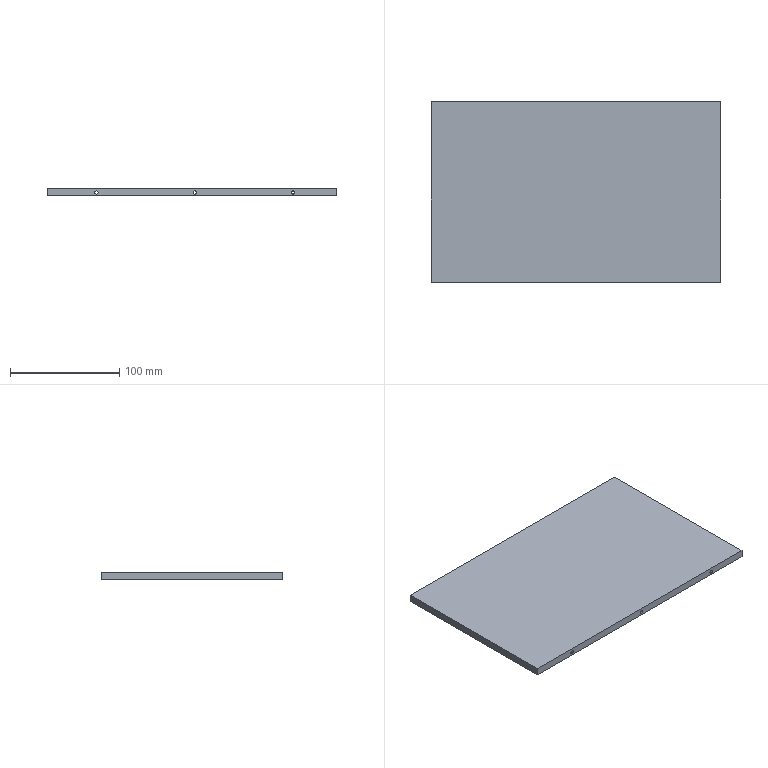Part | SolidWorks | features ICE 2, Extrusion 1, LPattern 1 | 1 solid | 23 faces | box 265 x 165 x 7 mm | volume 95885 mm3 | cylinder 12 | plane 11 | commonest cylinder face diameters 3 x12
STEP:
#1=CARTESIAN_POINT('',(135.,0.,-3.5));
#2=VERTEX_POINT('',#1);
#3=CARTESIAN_POINT('',(135.,0.,-0.5));
#4=VERTEX_POINT('',#3);
#5=CARTESIAN_POINT('',(135.,0.,-2.));
#6=DIRECTION('',(0.,1.,0.));
#7=DIRECTION('',(0.,0.,1.));
#8=AXIS2_PLACEMENT_3D('',#5,#6,#7);
#9=CIRCLE('',#8,1.5);
#10=EDGE_CURVE('',#2,#4,#9,.T.);
#11=ORIENTED_EDGE('',*,*,#10,.F.);
#12=CARTESIAN_POINT('',(135.,2.,-3.5));
#13=VERTEX_POINT('',#12);
#14=CARTESIAN_POINT('',(135.,0.,-3.5));
#15=DIRECTION('',(0.,1.,0.));
#16=VECTOR('',#15,1000.);
#17=LINE('',#14,#16);
#18=EDGE_CURVE('',#2,#13,#17,.T.);
#19=ORIENTED_EDGE('',*,*,#18,.T.);
#20=CARTESIAN_POINT('',(135.,2.,-0.5));
#21=VERTEX_POINT('',#20);
#22=CARTESIAN_POINT('',(135.,2.,-2.));
#23=DIRECTION('',(0.,1.,0.));
#24=DIRECTION('',(0.,0.,1.));
#25=AXIS2_PLACEMENT_3D('',#22,#23,#24);
#26=CIRCLE('',#25,1.5);
#27=EDGE_CURVE('',#13,#21,#26,.T.);
#28=ORIENTED_EDGE('',*,*,#27,.T.);
#29=CARTESIAN_POINT('',(135.,0.,-0.5));
#30=DIRECTION('',(0.,1.,0.));
#31=VECTOR('',#30,1000.);
#32=LINE('',#29,#31);
#33=EDGE_CURVE('',#4,#21,#32,.T.);
#34=ORIENTED_EDGE('',*,*,#33,.F.);
#35=EDGE_LOOP('',(#11,#19,#28,#34));
#36=FACE_OUTER_BOUND('',#35,.T.);
#37=CARTESIAN_POINT('',(135.,0.,-2.));
#38=DIRECTION('',(0.,1.,0.));
#39=DIRECTION('',(0.,0.,1.));
#40=AXIS2_PLACEMENT_3D('',#37,#38,#39);
#41=CYLINDRICAL_SURFACE('',#40,1.5);
#42=ADVANCED_FACE('',(#36),#41,.F.);
#43=CARTESIAN_POINT('',(135.,163.,-0.5));
#44=VERTEX_POINT('',#43);
#45=CARTESIAN_POINT('',(135.,163.,-3.5));
#46=VERTEX_POINT('',#45);
#47=CARTESIAN_POINT('',(135.,163.,-2.));
#48=DIRECTION('',(0.,-1.,0.));
#49=DIRECTION('',(0.,0.,-1.));
#50=AXIS2_PLACEMENT_3D('',#47,#48,#49);
#51=CIRCLE('',#50,1.5);
#52=EDGE_CURVE('',#44,#46,#51,.T.);
#53=ORIENTED_EDGE('',*,*,#52,.T.);
#54=CARTESIAN_POINT('',(135.,165.,-3.5));
#55=VERTEX_POINT('',#54);
#56=CARTESIAN_POINT('',(135.,0.,-3.5));
#57=DIRECTION('',(0.,1.,0.));
#58=VECTOR('',#57,1000.);
#59=LINE('',#56,#58);
#60=EDGE_CURVE('',#46,#55,#59,.T.);
#61=ORIENTED_EDGE('',*,*,#60,.T.);
#62=CARTESIAN_POINT('',(135.,165.,-0.5));
#63=VERTEX_POINT('',#62);
#64=CARTESIAN_POINT('',(135.,165.,-2.));
#65=DIRECTION('',(0.,1.,0.));
#66=DIRECTION('',(0.,0.,1.));
#67=AXIS2_PLACEMENT_3D('',#64,#65,#66);
#68=CIRCLE('',#67,1.5);
#69=EDGE_CURVE('',#55,#63,#68,.T.);
#70=ORIENTED_EDGE('',*,*,#69,.T.);
#71=CARTESIAN_POINT('',(135.,0.,-0.5));
#72=DIRECTION('',(0.,1.,0.));
#73=VECTOR('',#72,1000.);
#74=LINE('',#71,#73);
#75=EDGE_CURVE('',#44,#63,#74,.T.);
#76=ORIENTED_EDGE('',*,*,#75,.F.);
#77=EDGE_LOOP('',(#53,#61,#70,#76));
#78=FACE_OUTER_BOUND('',#77,.T.);
#79=CARTESIAN_POINT('',(135.,0.,-2.));
#80=DIRECTION('',(0.,1.,0.));
#81=DIRECTION('',(0.,0.,1.));
#82=AXIS2_PLACEMENT_3D('',#79,#80,#81);
#83=CYLINDRICAL_SURFACE('',#82,1.5);
#84=ADVANCED_FACE('',(#78),#83,.F.);
#85=CARTESIAN_POINT('',(225.,163.,-0.5));
#86=VERTEX_POINT('',#85);
#87=CARTESIAN_POINT('',(225.,163.,-3.5));
#88=VERTEX_POINT('',#87);
#89=CARTESIAN_POINT('',(225.,163.,-2.));
#90=DIRECTION('',(0.,-1.,0.));
#91=DIRECTION('',(0.,0.,-1.));
#92=AXIS2_PLACEMENT_3D('',#89,#90,#91);
#93=CIRCLE('',#92,1.5);
#94=EDGE_CURVE('',#86,#88,#93,.T.);
#95=ORIENTED_EDGE('',*,*,#94,.T.);
#96=CARTESIAN_POINT('',(225.,165.,-3.5));
#97=VERTEX_POINT('',#96);
#98=CARTESIAN_POINT('',(225.,0.,-3.5));
#99=DIRECTION('',(0.,1.,0.));
#100=VECTOR('',#99,1000.);
#101=LINE('',#98,#100);
#102=EDGE_CURVE('',#88,#97,#101,.T.);
#103=ORIENTED_EDGE('',*,*,#102,.T.);
#104=CARTESIAN_POINT('',(225.,165.,-0.5));
#105=VERTEX_POINT('',#104);
#106=CARTESIAN_POINT('',(225.,165.,-2.));
#107=DIRECTION('',(0.,1.,0.));
#108=DIRECTION('',(0.,0.,1.));
#109=AXIS2_PLACEMENT_3D('',#106,#107,#108);
#110=CIRCLE('',#109,1.5);
#111=EDGE_CURVE('',#97,#105,#110,.T.);
#112=ORIENTED_EDGE('',*,*,#111,.T.);
#113=CARTESIAN_POINT('',(225.,0.,-0.5));
#114=DIRECTION('',(0.,1.,0.));
#115=VECTOR('',#114,1000.);
#116=LINE('',#113,#115);
#117=EDGE_CURVE('',#86,#105,#116,.T.);
#118=ORIENTED_EDGE('',*,*,#117,.F.);
#119=EDGE_LOOP('',(#95,#103,#112,#118));
#120=FACE_OUTER_BOUND('',#119,.T.);
#121=CARTESIAN_POINT('',(225.,0.,-2.));
#122=DIRECTION('',(0.,1.,0.));
#123=DIRECTION('',(0.,0.,1.));
#124=AXIS2_PLACEMENT_3D('',#121,#122,#123);
#125=CYLINDRICAL_SURFACE('',#124,1.5);
#126=ADVANCED_FACE('',(#120),#125,.F.);
#127=CARTESIAN_POINT('',(225.,0.,-3.5));
#128=VERTEX_POINT('',#127);
#129=CARTESIAN_POINT('',(225.,0.,-0.5));
#130=VERTEX_POINT('',#129);
#131=CARTESIAN_POINT('',(225.,0.,-2.));
#132=DIRECTION('',(0.,1.,0.));
#133=DIRECTION('',(0.,0.,1.));
#134=AXIS2_PLACEMENT_3D('',#131,#132,#133);
#135=CIRCLE('',#134,1.5);
#136=EDGE_CURVE('',#128,#130,#135,.T.);
#137=ORIENTED_EDGE('',*,*,#136,.F.);
#138=CARTESIAN_POINT('',(225.,2.,-3.5));
#139=VERTEX_POINT('',#138);
#140=CARTESIAN_POINT('',(225.,0.,-3.5));
#141=DIRECTION('',(0.,1.,0.));
#142=VECTOR('',#141,1000.);
#143=LINE('',#140,#142);
#144=EDGE_CURVE('',#128,#139,#143,.T.);
#145=ORIENTED_EDGE('',*,*,#144,.T.);
#146=CARTESIAN_POINT('',(225.,2.,-0.5));
#147=VERTEX_POINT('',#146);
#148=CARTESIAN_POINT('',(225.,2.,-2.));
#149=DIRECTION('',(0.,1.,0.));
#150=DIRECTION('',(0.,0.,1.));
#151=AXIS2_PLACEMENT_3D('',#148,#149,#150);
#152=CIRCLE('',#151,1.5);
#153=EDGE_CURVE('',#139,#147,#152,.T.);
#154=ORIENTED_EDGE('',*,*,#153,.T.);
#155=CARTESIAN_POINT('',(225.,0.,-0.5));
#156=DIRECTION('',(0.,1.,0.));
#157=VECTOR('',#156,1000.);
#158=LINE('',#155,#157);
#159=EDGE_CURVE('',#130,#147,#158,.T.);
#160=ORIENTED_EDGE('',*,*,#159,.F.);
#161=EDGE_LOOP('',(#137,#145,#154,#160));
#162=FACE_OUTER_BOUND('',#161,.T.);
#163=CARTESIAN_POINT('',(225.,0.,-2.));
#164=DIRECTION('',(0.,1.,0.));
#165=DIRECTION('',(0.,0.,1.));
#166=AXIS2_PLACEMENT_3D('',#163,#164,#165);
#167=CYLINDRICAL_SURFACE('',#166,1.5);
#168=ADVANCED_FACE('',(#162),#167,.F.);
#169=CARTESIAN_POINT('',(45.,163.,-0.5));
#170=VERTEX_POINT('',#169);
#171=CARTESIAN_POINT('',(45.,163.,-3.5));
#172=VERTEX_POINT('',#171);
#173=CARTESIAN_POINT('',(45.,163.,-2.));
#174=DIRECTION('',(0.,-1.,0.));
#175=DIRECTION('',(0.,0.,-1.));
#176=AXIS2_PLACEMENT_3D('',#173,#174,#175);
#177=CIRCLE('',#176,1.5);
#178=EDGE_CURVE('',#170,#172,#177,.T.);
#179=ORIENTED_EDGE('',*,*,#178,.T.);
#180=CARTESIAN_POINT('',(45.,165.,-3.5));
#181=VERTEX_POINT('',#180);
#182=CARTESIAN_POINT('',(45.,0.,-3.5));
#183=DIRECTION('',(0.,1.,0.));
#184=VECTOR('',#183,1000.);
#185=LINE('',#182,#184);
#186=EDGE_CURVE('',#172,#181,#185,.T.);
#187=ORIENTED_EDGE('',*,*,#186,.T.);
#188=CARTESIAN_POINT('',(45.,165.,-0.5));
#189=VERTEX_POINT('',#188);
#190=CARTESIAN_POINT('',(45.,165.,-2.));
#191=DIRECTION('',(0.,1.,0.));
#192=DIRECTION('',(0.,0.,1.));
#193=AXIS2_PLACEMENT_3D('',#190,#191,#192);
#194=CIRCLE('',#193,1.5);
#195=EDGE_CURVE('',#181,#189,#194,.T.);
#196=ORIENTED_EDGE('',*,*,#195,.T.);
#197=CARTESIAN_POINT('',(45.,0.,-0.5));
#198=DIRECTION('',(0.,1.,0.));
#199=VECTOR('',#198,1000.);
#200=LINE('',#197,#199);
#201=EDGE_CURVE('',#170,#189,#200,.T.);
#202=ORIENTED_EDGE('',*,*,#201,.F.);
#203=EDGE_LOOP('',(#179,#187,#196,#202));
#204=FACE_OUTER_BOUND('',#203,.T.);
#205=CARTESIAN_POINT('',(45.,0.,-2.));
#206=DIRECTION('',(0.,1.,0.));
#207=DIRECTION('',(0.,0.,1.));
#208=AXIS2_PLACEMENT_3D('',#205,#206,#207);
#209=CYLINDRICAL_SURFACE('',#208,1.5);
#210=ADVANCED_FACE('',(#204),#209,.F.);
#211=CARTESIAN_POINT('',(45.,0.,-3.5));
#212=VERTEX_POINT('',#211);
#213=CARTESIAN_POINT('',(45.,0.,-0.5));
#214=VERTEX_POINT('',#213);
#215=CARTESIAN_POINT('',(45.,0.,-2.));
#216=DIRECTION('',(0.,1.,0.));
#217=DIRECTION('',(0.,0.,1.));
#218=AXIS2_PLACEMENT_3D('',#215,#216,#217);
#219=CIRCLE('',#218,1.5);
#220=EDGE_CURVE('',#212,#214,#219,.T.);
#221=ORIENTED_EDGE('',*,*,#220,.F.);
#222=CARTESIAN_POINT('',(45.,2.,-3.5));
#223=VERTEX_POINT('',#222);
#224=CARTESIAN_POINT('',(45.,0.,-3.5));
#225=DIRECTION('',(0.,1.,0.));
#226=VECTOR('',#225,1000.);
#227=LINE('',#224,#226);
#228=EDGE_CURVE('',#212,#223,#227,.T.);
#229=ORIENTED_EDGE('',*,*,#228,.T.);
#230=CARTESIAN_POINT('',(45.,2.,-0.5));
#231=VERTEX_POINT('',#230);
#232=CARTESIAN_POINT('',(45.,2.,-2.));
#233=DIRECTION('',(0.,1.,0.));
#234=DIRECTION('',(0.,0.,1.));
#235=AXIS2_PLACEMENT_3D('',#232,#233,#234);
#236=CIRCLE('',#235,1.5);
#237=EDGE_CURVE('',#223,#231,#236,.T.);
#238=ORIENTED_EDGE('',*,*,#237,.T.);
#239=CARTESIAN_POINT('',(45.,0.,-0.5));
#240=DIRECTION('',(0.,1.,0.));
#241=VECTOR('',#240,1000.);
#242=LINE('',#239,#241);
#243=EDGE_CURVE('',#214,#231,#242,.T.);
#244=ORIENTED_EDGE('',*,*,#243,.F.);
#245=EDGE_LOOP('',(#221,#229,#238,#244));
#246=FACE_OUTER_BOUND('',#245,.T.);
#247=CARTESIAN_POINT('',(45.,0.,-2.));
#248=DIRECTION('',(0.,1.,0.));
#249=DIRECTION('',(0.,0.,1.));
#250=AXIS2_PLACEMENT_3D('',#247,#248,#249);
#251=CYLINDRICAL_SURFACE('',#250,1.5);
#252=ADVANCED_FACE('',(#246),#251,.F.);
#253=ORIENTED_EDGE('',*,*,#228,.F.);
#254=CARTESIAN_POINT('',(45.,0.,-2.));
#255=DIRECTION('',(0.,1.,0.));
#256=DIRECTION('',(0.,0.,1.));
#257=AXIS2_PLACEMENT_3D('',#254,#255,#256);
#258=CIRCLE('',#257,1.5);
#259=EDGE_CURVE('',#214,#212,#258,.T.);
#260=ORIENTED_EDGE('',*,*,#259,.F.);
#261=ORIENTED_EDGE('',*,*,#243,.T.);
#262=CARTESIAN_POINT('',(45.,2.,-2.));
#263=DIRECTION('',(0.,1.,0.));
#264=DIRECTION('',(0.,0.,1.));
#265=AXIS2_PLACEMENT_3D('',#262,#263,#264);
#266=CIRCLE('',#265,1.5);
#267=EDGE_CURVE('',#231,#223,#266,.T.);
#268=ORIENTED_EDGE('',*,*,#267,.T.);
#269=EDGE_LOOP('',(#253,#260,#261,#268));
#270=FACE_OUTER_BOUND('',#269,.T.);
#271=CARTESIAN_POINT('',(45.,0.,-2.));
#272=DIRECTION('',(0.,1.,0.));
#273=DIRECTION('',(0.,0.,1.));
#274=AXIS2_PLACEMENT_3D('',#271,#272,#273);
#275=CYLINDRICAL_SURFACE('',#274,1.5);
#276=ADVANCED_FACE('',(#270),#275,.F.);
#277=ORIENTED_EDGE('',*,*,#186,.F.);
#278=CARTESIAN_POINT('',(45.,163.,-2.));
#279=DIRECTION('',(0.,-1.,0.));
#280=DIRECTION('',(0.,0.,-1.));
#281=AXIS2_PLACEMENT_3D('',#278,#279,#280);
#282=CIRCLE('',#281,1.5);
#283=EDGE_CURVE('',#172,#170,#282,.T.);
#284=ORIENTED_EDGE('',*,*,#283,.T.);
#285=ORIENTED_EDGE('',*,*,#201,.T.);
#286=CARTESIAN_POINT('',(45.,165.,-2.));
#287=DIRECTION('',(0.,1.,0.));
#288=DIRECTION('',(0.,0.,1.));
#289=AXIS2_PLACEMENT_3D('',#286,#287,#288);
#290=CIRCLE('',#289,1.5);
#291=EDGE_CURVE('',#189,#181,#290,.T.);
#292=ORIENTED_EDGE('',*,*,#291,.T.);
#293=EDGE_LOOP('',(#277,#284,#285,#292));
#294=FACE_OUTER_BOUND('',#293,.T.);
#295=CARTESIAN_POINT('',(45.,0.,-2.));
#296=DIRECTION('',(0.,1.,0.));
#297=DIRECTION('',(0.,0.,1.));
#298=AXIS2_PLACEMENT_3D('',#295,#296,#297);
#299=CYLINDRICAL_SURFACE('',#298,1.5);
#300=ADVANCED_FACE('',(#294),#299,.F.);
#301=CARTESIAN_POINT('',(0.,165.,2.));
#302=VERTEX_POINT('',#301);
#303=CARTESIAN_POINT('',(0.,165.,-5.));
#304=VERTEX_POINT('',#303);
#305=CARTESIAN_POINT('',(0.,165.,2.));
#306=DIRECTION('',(0.,0.,-1.));
#307=VECTOR('',#306,1000.);
#308=LINE('',#305,#307);
#309=EDGE_CURVE('',#302,#304,#308,.T.);
#310=ORIENTED_EDGE('',*,*,#309,.T.);
#311=CARTESIAN_POINT('',(0.,0.,-5.));
#312=VERTEX_POINT('',#311);
#313=CARTESIAN_POINT('',(0.,0.,-5.));
#314=DIRECTION('',(0.,1.,0.));
#315=VECTOR('',#314,1000.);
#316=LINE('',#313,#315);
#317=EDGE_CURVE('',#312,#304,#316,.T.);
#318=ORIENTED_EDGE('',*,*,#317,.F.);
#319=CARTESIAN_POINT('',(0.,0.,2.));
#320=VERTEX_POINT('',#319);
#321=CARTESIAN_POINT('',(0.,0.,2.));
#322=DIRECTION('',(0.,0.,-1.));
#323=VECTOR('',#322,1000.);
#324=LINE('',#321,#323);
#325=EDGE_CURVE('',#320,#312,#324,.T.);
#326=ORIENTED_EDGE('',*,*,#325,.F.);
#327=CARTESIAN_POINT('',(0.,0.,2.));
#328=DIRECTION('',(0.,-1.,0.));
#329=VECTOR('',#328,1000.);
#330=LINE('',#327,#329);
#331=EDGE_CURVE('',#302,#320,#330,.T.);
#332=ORIENTED_EDGE('',*,*,#331,.F.);
#333=EDGE_LOOP('',(#310,#318,#326,#332));
#334=FACE_OUTER_BOUND('',#333,.T.);
#335=CARTESIAN_POINT('',(0.,0.,2.));
#336=DIRECTION('',(1.,0.,0.));
#337=DIRECTION('',(0.,0.,-1.));
#338=AXIS2_PLACEMENT_3D('',#335,#336,#337);
#339=PLANE('',#338);
#340=ADVANCED_FACE('',(#334),#339,.F.);
#341=CARTESIAN_POINT('',(135.,0.,-2.));
#342=DIRECTION('',(0.,1.,0.));
#343=DIRECTION('',(0.,0.,1.));
#344=AXIS2_PLACEMENT_3D('',#341,#342,#343);
#345=CIRCLE('',#344,1.5);
#346=EDGE_CURVE('',#4,#2,#345,.T.);
#347=ORIENTED_EDGE('',*,*,#346,.T.);
#348=ORIENTED_EDGE('',*,*,#10,.T.);
#349=EDGE_LOOP('',(#347,#348));
#350=FACE_BOUND('',#349,.T.);
#351=CARTESIAN_POINT('',(225.,0.,-2.));
#352=DIRECTION('',(0.,1.,0.));
#353=DIRECTION('',(0.,0.,1.));
#354=AXIS2_PLACEMENT_3D('',#351,#352,#353);
#355=CIRCLE('',#354,1.5);
#356=EDGE_CURVE('',#130,#128,#355,.T.);
#357=ORIENTED_EDGE('',*,*,#356,.T.);
#358=ORIENTED_EDGE('',*,*,#136,.T.);
#359=EDGE_LOOP('',(#357,#358));
#360=FACE_BOUND('',#359,.T.);
#361=ORIENTED_EDGE('',*,*,#325,.T.);
#362=CARTESIAN_POINT('',(265.,0.,-5.));
#363=VERTEX_POINT('',#362);
#364=CARTESIAN_POINT('',(265.,0.,-5.));
#365=DIRECTION('',(-1.,0.,0.));
#366=VECTOR('',#365,1000.);
#367=LINE('',#364,#366);
#368=EDGE_CURVE('',#363,#312,#367,.T.);
#369=ORIENTED_EDGE('',*,*,#368,.F.);
#370=CARTESIAN_POINT('',(265.,0.,2.));
#371=VERTEX_POINT('',#370);
#372=CARTESIAN_POINT('',(265.,0.,2.));
#373=DIRECTION('',(0.,0.,-1.));
#374=VECTOR('',#373,1000.);
#375=LINE('',#372,#374);
#376=EDGE_CURVE('',#371,#363,#375,.T.);
#377=ORIENTED_EDGE('',*,*,#376,.F.);
#378=CARTESIAN_POINT('',(0.,0.,2.));
#379=DIRECTION('',(1.,0.,0.));
#380=VECTOR('',#379,1000.);
#381=LINE('',#378,#380);
#382=EDGE_CURVE('',#320,#371,#381,.T.);
#383=ORIENTED_EDGE('',*,*,#382,.F.);
#384=EDGE_LOOP('',(#361,#369,#377,#383));
#385=FACE_OUTER_BOUND('',#384,.T.);
#386=ORIENTED_EDGE('',*,*,#259,.T.);
#387=ORIENTED_EDGE('',*,*,#220,.T.);
#388=EDGE_LOOP('',(#386,#387));
#389=FACE_BOUND('',#388,.T.);
#390=CARTESIAN_POINT('',(0.,0.,2.));
#391=DIRECTION('',(0.,1.,0.));
#392=DIRECTION('',(0.,0.,1.));
#393=AXIS2_PLACEMENT_3D('',#390,#391,#392);
#394=PLANE('',#393);
#395=ADVANCED_FACE('',(#350,#360,#385,#389),#394,.F.);
#396=ORIENTED_EDGE('',*,*,#376,.T.);
#397=CARTESIAN_POINT('',(265.,165.,-5.));
#398=VERTEX_POINT('',#397);
#399=CARTESIAN_POINT('',(265.,165.,-5.));
#400=DIRECTION('',(0.,-1.,0.));
#401=VECTOR('',#400,1000.);
#402=LINE('',#399,#401);
#403=EDGE_CURVE('',#398,#363,#402,.T.);
#404=ORIENTED_EDGE('',*,*,#403,.F.);
#405=CARTESIAN_POINT('',(265.,165.,2.));
#406=VERTEX_POINT('',#405);
#407=CARTESIAN_POINT('',(265.,165.,2.));
#408=DIRECTION('',(0.,0.,-1.));
#409=VECTOR('',#408,1000.);
#410=LINE('',#407,#409);
#411=EDGE_CURVE('',#406,#398,#410,.T.);
#412=ORIENTED_EDGE('',*,*,#411,.F.);
#413=CARTESIAN_POINT('',(265.,0.,2.));
#414=DIRECTION('',(0.,1.,0.));
#415=VECTOR('',#414,1000.);
#416=LINE('',#413,#415);
#417=EDGE_CURVE('',#371,#406,#416,.T.);
#418=ORIENTED_EDGE('',*,*,#417,.F.);
#419=EDGE_LOOP('',(#396,#404,#412,#418));
#420=FACE_OUTER_BOUND('',#419,.T.);
#421=CARTESIAN_POINT('',(265.,0.,2.));
#422=DIRECTION('',(-1.,0.,0.));
#423=DIRECTION('',(0.,0.,1.));
#424=AXIS2_PLACEMENT_3D('',#421,#422,#423);
#425=PLANE('',#424);
#426=ADVANCED_FACE('',(#420),#425,.F.);
#427=CARTESIAN_POINT('',(135.,165.,-2.));
#428=DIRECTION('',(0.,1.,0.));
#429=DIRECTION('',(0.,0.,1.));
#430=AXIS2_PLACEMENT_3D('',#427,#428,#429);
#431=CIRCLE('',#430,1.5);
#432=EDGE_CURVE('',#63,#55,#431,.T.);
#433=ORIENTED_EDGE('',*,*,#432,.F.);
#434=ORIENTED_EDGE('',*,*,#69,.F.);
#435=EDGE_LOOP('',(#433,#434));
#436=FACE_BOUND('',#435,.T.);
#437=CARTESIAN_POINT('',(225.,165.,-2.));
#438=DIRECTION('',(0.,1.,0.));
#439=DIRECTION('',(0.,0.,1.));
#440=AXIS2_PLACEMENT_3D('',#437,#438,#439);
#441=CIRCLE('',#440,1.5);
#442=EDGE_CURVE('',#105,#97,#441,.T.);
#443=ORIENTED_EDGE('',*,*,#442,.F.);
#444=ORIENTED_EDGE('',*,*,#111,.F.);
#445=EDGE_LOOP('',(#443,#444));
#446=FACE_BOUND('',#445,.T.);
#447=ORIENTED_EDGE('',*,*,#411,.T.);
#448=CARTESIAN_POINT('',(0.,165.,-5.));
#449=DIRECTION('',(1.,0.,0.));
#450=VECTOR('',#449,1000.);
#451=LINE('',#448,#450);
#452=EDGE_CURVE('',#304,#398,#451,.T.);
#453=ORIENTED_EDGE('',*,*,#452,.F.);
#454=ORIENTED_EDGE('',*,*,#309,.F.);
#455=CARTESIAN_POINT('',(0.,165.,2.));
#456=DIRECTION('',(-1.,0.,0.));
#457=VECTOR('',#456,1000.);
#458=LINE('',#455,#457);
#459=EDGE_CURVE('',#406,#302,#458,.T.);
#460=ORIENTED_EDGE('',*,*,#459,.F.);
#461=EDGE_LOOP('',(#447,#453,#454,#460));
#462=FACE_OUTER_BOUND('',#461,.T.);
#463=ORIENTED_EDGE('',*,*,#291,.F.);
#464=ORIENTED_EDGE('',*,*,#195,.F.);
#465=EDGE_LOOP('',(#463,#464));
#466=FACE_BOUND('',#465,.T.);
#467=CARTESIAN_POINT('',(0.,165.,2.));
#468=DIRECTION('',(0.,-1.,0.));
#469=DIRECTION('',(0.,0.,-1.));
#470=AXIS2_PLACEMENT_3D('',#467,#468,#469);
#471=PLANE('',#470);
#472=ADVANCED_FACE('',(#436,#446,#462,#466),#471,.F.);
#473=ORIENTED_EDGE('',*,*,#331,.T.);
#474=ORIENTED_EDGE('',*,*,#382,.T.);
#475=ORIENTED_EDGE('',*,*,#417,.T.);
#476=ORIENTED_EDGE('',*,*,#459,.T.);
#477=EDGE_LOOP('',(#473,#474,#475,#476));
#478=FACE_OUTER_BOUND('',#477,.T.);
#479=CARTESIAN_POINT('',(0.,0.,2.));
#480=DIRECTION('',(0.,0.,-1.));
#481=DIRECTION('',(-1.,0.,0.));
#482=AXIS2_PLACEMENT_3D('',#479,#480,#481);
#483=PLANE('',#482);
#484=ADVANCED_FACE('',(#478),#483,.F.);
#485=ORIENTED_EDGE('',*,*,#368,.T.);
#486=ORIENTED_EDGE('',*,*,#317,.T.);
#487=ORIENTED_EDGE('',*,*,#452,.T.);
#488=ORIENTED_EDGE('',*,*,#403,.T.);
#489=EDGE_LOOP('',(#485,#486,#487,#488));
#490=FACE_OUTER_BOUND('',#489,.T.);
#491=CARTESIAN_POINT('',(2.,163.,-5.));
#492=VERTEX_POINT('',#491);
#493=CARTESIAN_POINT('',(263.,163.,-5.));
#494=VERTEX_POINT('',#493);
#495=CARTESIAN_POINT('',(2.,163.,-5.));
#496=DIRECTION('',(1.,0.,0.));
#497=VECTOR('',#496,1000.);
#498=LINE('',#495,#497);
#499=EDGE_CURVE('',#492,#494,#498,.T.);
#500=ORIENTED_EDGE('',*,*,#499,.F.);
#501=CARTESIAN_POINT('',(2.,2.,-5.));
#502=VERTEX_POINT('',#501);
#503=CARTESIAN_POINT('',(2.,2.,-5.));
#504=DIRECTION('',(0.,1.,0.));
#505=VECTOR('',#504,1000.);
#506=LINE('',#503,#505);
#507=EDGE_CURVE('',#502,#492,#506,.T.);
#508=ORIENTED_EDGE('',*,*,#507,.F.);
#509=CARTESIAN_POINT('',(263.,2.,-5.));
#510=VERTEX_POINT('',#509);
#511=CARTESIAN_POINT('',(263.,2.,-5.));
#512=DIRECTION('',(-1.,0.,0.));
#513=VECTOR('',#512,1000.);
#514=LINE('',#511,#513);
#515=EDGE_CURVE('',#510,#502,#514,.T.);
#516=ORIENTED_EDGE('',*,*,#515,.F.);
#517=CARTESIAN_POINT('',(263.,163.,-5.));
#518=DIRECTION('',(0.,-1.,0.));
#519=VECTOR('',#518,1000.);
#520=LINE('',#517,#519);
#521=EDGE_CURVE('',#494,#510,#520,.T.);
#522=ORIENTED_EDGE('',*,*,#521,.F.);
#523=EDGE_LOOP('',(#500,#508,#516,#522));
#524=FACE_BOUND('',#523,.T.);
#525=CARTESIAN_POINT('',(0.,0.,-5.));
#526=DIRECTION('',(0.,0.,-1.));
#527=DIRECTION('',(-1.,0.,0.));
#528=AXIS2_PLACEMENT_3D('',#525,#526,#527);
#529=PLANE('',#528);
#530=ADVANCED_FACE('',(#490,#524),#529,.T.);
#531=CARTESIAN_POINT('',(2.,2.,0.));
#532=VERTEX_POINT('',#531);
#533=CARTESIAN_POINT('',(2.,163.,0.));
#534=VERTEX_POINT('',#533);
#535=CARTESIAN_POINT('',(2.,2.,0.));
#536=DIRECTION('',(0.,1.,0.));
#537=VECTOR('',#536,1000.);
#538=LINE('',#535,#537);
#539=EDGE_CURVE('',#532,#534,#538,.T.);
#540=ORIENTED_EDGE('',*,*,#539,.F.);
#541=CARTESIAN_POINT('',(2.,2.,-5.));
#542=DIRECTION('',(0.,0.,1.));
#543=VECTOR('',#542,1000.);
#544=LINE('',#541,#543);
#545=EDGE_CURVE('',#502,#532,#544,.T.);
#546=ORIENTED_EDGE('',*,*,#545,.F.);
#547=ORIENTED_EDGE('',*,*,#507,.T.);
#548=CARTESIAN_POINT('',(2.,163.,-5.));
#549=DIRECTION('',(0.,0.,1.));
#550=VECTOR('',#549,1000.);
#551=LINE('',#548,#550);
#552=EDGE_CURVE('',#492,#534,#551,.T.);
#553=ORIENTED_EDGE('',*,*,#552,.T.);
#554=EDGE_LOOP('',(#540,#546,#547,#553));
#555=FACE_OUTER_BOUND('',#554,.T.);
#556=CARTESIAN_POINT('',(2.,2.,-5.));
#557=DIRECTION('',(1.,0.,0.));
#558=DIRECTION('',(0.,0.,-1.));
#559=AXIS2_PLACEMENT_3D('',#556,#557,#558);
#560=PLANE('',#559);
#561=ADVANCED_FACE('',(#555),#560,.T.);
#562=ORIENTED_EDGE('',*,*,#52,.F.);
#563=CARTESIAN_POINT('',(135.,163.,-2.));
#564=DIRECTION('',(0.,-1.,0.));
#565=DIRECTION('',(0.,0.,-1.));
#566=AXIS2_PLACEMENT_3D('',#563,#564,#565);
#567=CIRCLE('',#566,1.5);
#568=EDGE_CURVE('',#46,#44,#567,.T.);
#569=ORIENTED_EDGE('',*,*,#568,.F.);
#570=EDGE_LOOP('',(#562,#569));
#571=FACE_BOUND('',#570,.T.);
#572=ORIENTED_EDGE('',*,*,#94,.F.);
#573=CARTESIAN_POINT('',(225.,163.,-2.));
#574=DIRECTION('',(0.,-1.,0.));
#575=DIRECTION('',(0.,0.,-1.));
#576=AXIS2_PLACEMENT_3D('',#573,#574,#575);
#577=CIRCLE('',#576,1.5);
#578=EDGE_CURVE('',#88,#86,#577,.T.);
#579=ORIENTED_EDGE('',*,*,#578,.F.);
#580=EDGE_LOOP('',(#572,#579));
#581=FACE_BOUND('',#580,.T.);
#582=CARTESIAN_POINT('',(263.,163.,0.));
#583=VERTEX_POINT('',#582);
#584=CARTESIAN_POINT('',(2.,163.,0.));
#585=DIRECTION('',(1.,0.,0.));
#586=VECTOR('',#585,1000.);
#587=LINE('',#584,#586);
#588=EDGE_CURVE('',#534,#583,#587,.T.);
#589=ORIENTED_EDGE('',*,*,#588,.F.);
#590=ORIENTED_EDGE('',*,*,#552,.F.);
#591=ORIENTED_EDGE('',*,*,#499,.T.);
#592=CARTESIAN_POINT('',(263.,163.,-5.));
#593=DIRECTION('',(0.,0.,1.));
#594=VECTOR('',#593,1000.);
#595=LINE('',#592,#594);
#596=EDGE_CURVE('',#494,#583,#595,.T.);
#597=ORIENTED_EDGE('',*,*,#596,.T.);
#598=EDGE_LOOP('',(#589,#590,#591,#597));
#599=FACE_OUTER_BOUND('',#598,.T.);
#600=ORIENTED_EDGE('',*,*,#178,.F.);
#601=ORIENTED_EDGE('',*,*,#283,.F.);
#602=EDGE_LOOP('',(#600,#601));
#603=FACE_BOUND('',#602,.T.);
#604=CARTESIAN_POINT('',(2.,163.,-5.));
#605=DIRECTION('',(0.,-1.,0.));
#606=DIRECTION('',(0.,0.,-1.));
#607=AXIS2_PLACEMENT_3D('',#604,#605,#606);
#608=PLANE('',#607);
#609=ADVANCED_FACE('',(#571,#581,#599,#603),#608,.T.);
#610=CARTESIAN_POINT('',(263.,2.,0.));
#611=VERTEX_POINT('',#610);
#612=CARTESIAN_POINT('',(263.,163.,0.));
#613=DIRECTION('',(0.,-1.,0.));
#614=VECTOR('',#613,1000.);
#615=LINE('',#612,#614);
#616=EDGE_CURVE('',#583,#611,#615,.T.);
#617=ORIENTED_EDGE('',*,*,#616,.F.);
#618=ORIENTED_EDGE('',*,*,#596,.F.);
#619=ORIENTED_EDGE('',*,*,#521,.T.);
#620=CARTESIAN_POINT('',(263.,2.,-5.));
#621=DIRECTION('',(0.,0.,1.));
#622=VECTOR('',#621,1000.);
#623=LINE('',#620,#622);
#624=EDGE_CURVE('',#510,#611,#623,.T.);
#625=ORIENTED_EDGE('',*,*,#624,.T.);
#626=EDGE_LOOP('',(#617,#618,#619,#625));
#627=FACE_OUTER_BOUND('',#626,.T.);
#628=CARTESIAN_POINT('',(263.,163.,-5.));
#629=DIRECTION('',(-1.,0.,0.));
#630=DIRECTION('',(0.,0.,1.));
#631=AXIS2_PLACEMENT_3D('',#628,#629,#630);
#632=PLANE('',#631);
#633=ADVANCED_FACE('',(#627),#632,.T.);
#634=CARTESIAN_POINT('',(135.,2.,-2.));
#635=DIRECTION('',(0.,1.,0.));
#636=DIRECTION('',(0.,0.,1.));
#637=AXIS2_PLACEMENT_3D('',#634,#635,#636);
#638=CIRCLE('',#637,1.5);
#639=EDGE_CURVE('',#21,#13,#638,.T.);
#640=ORIENTED_EDGE('',*,*,#639,.F.);
#641=ORIENTED_EDGE('',*,*,#27,.F.);
#642=EDGE_LOOP('',(#640,#641));
#643=FACE_BOUND('',#642,.T.);
#644=CARTESIAN_POINT('',(225.,2.,-2.));
#645=DIRECTION('',(0.,1.,0.));
#646=DIRECTION('',(0.,0.,1.));
#647=AXIS2_PLACEMENT_3D('',#644,#645,#646);
#648=CIRCLE('',#647,1.5);
#649=EDGE_CURVE('',#147,#139,#648,.T.);
#650=ORIENTED_EDGE('',*,*,#649,.F.);
#651=ORIENTED_EDGE('',*,*,#153,.F.);
#652=EDGE_LOOP('',(#650,#651));
#653=FACE_BOUND('',#652,.T.);
#654=CARTESIAN_POINT('',(263.,2.,0.));
#655=DIRECTION('',(-1.,0.,0.));
#656=VECTOR('',#655,1000.);
#657=LINE('',#654,#656);
#658=EDGE_CURVE('',#611,#532,#657,.T.);
#659=ORIENTED_EDGE('',*,*,#658,.F.);
#660=ORIENTED_EDGE('',*,*,#624,.F.);
#661=ORIENTED_EDGE('',*,*,#515,.T.);
#662=ORIENTED_EDGE('',*,*,#545,.T.);
#663=EDGE_LOOP('',(#659,#660,#661,#662));
#664=FACE_OUTER_BOUND('',#663,.T.);
#665=ORIENTED_EDGE('',*,*,#267,.F.);
#666=ORIENTED_EDGE('',*,*,#237,.F.);
#667=EDGE_LOOP('',(#665,#666));
#668=FACE_BOUND('',#667,.T.);
#669=CARTESIAN_POINT('',(263.,2.,-5.));
#670=DIRECTION('',(0.,1.,0.));
#671=DIRECTION('',(0.,0.,1.));
#672=AXIS2_PLACEMENT_3D('',#669,#670,#671);
#673=PLANE('',#672);
#674=ADVANCED_FACE('',(#643,#653,#664,#668),#673,.T.);
#675=ORIENTED_EDGE('',*,*,#539,.T.);
#676=ORIENTED_EDGE('',*,*,#588,.T.);
#677=ORIENTED_EDGE('',*,*,#616,.T.);
#678=ORIENTED_EDGE('',*,*,#658,.T.);
#679=EDGE_LOOP('',(#675,#676,#677,#678));
#680=FACE_OUTER_BOUND('',#679,.T.);
#681=CARTESIAN_POINT('',(0.,0.,0.));
#682=DIRECTION('',(0.,0.,-1.));
#683=DIRECTION('',(-1.,0.,0.));
#684=AXIS2_PLACEMENT_3D('',#681,#682,#683);
#685=PLANE('',#684);
#686=ADVANCED_FACE('',(#680),#685,.T.);
#687=ORIENTED_EDGE('',*,*,#144,.F.);
#688=ORIENTED_EDGE('',*,*,#356,.F.);
#689=ORIENTED_EDGE('',*,*,#159,.T.);
#690=ORIENTED_EDGE('',*,*,#649,.T.);
#691=EDGE_LOOP('',(#687,#688,#689,#690));
#692=FACE_OUTER_BOUND('',#691,.T.);
#693=CARTESIAN_POINT('',(225.,0.,-2.));
#694=DIRECTION('',(0.,1.,0.));
#695=DIRECTION('',(0.,0.,1.));
#696=AXIS2_PLACEMENT_3D('',#693,#694,#695);
#697=CYLINDRICAL_SURFACE('',#696,1.5);
#698=ADVANCED_FACE('',(#692),#697,.F.);
#699=ORIENTED_EDGE('',*,*,#102,.F.);
#700=ORIENTED_EDGE('',*,*,#578,.T.);
#701=ORIENTED_EDGE('',*,*,#117,.T.);
#702=ORIENTED_EDGE('',*,*,#442,.T.);
#703=EDGE_LOOP('',(#699,#700,#701,#702));
#704=FACE_OUTER_BOUND('',#703,.T.);
#705=CARTESIAN_POINT('',(225.,0.,-2.));
#706=DIRECTION('',(0.,1.,0.));
#707=DIRECTION('',(0.,0.,1.));
#708=AXIS2_PLACEMENT_3D('',#705,#706,#707);
#709=CYLINDRICAL_SURFACE('',#708,1.5);
#710=ADVANCED_FACE('',(#704),#709,.F.);
#711=ORIENTED_EDGE('',*,*,#60,.F.);
#712=ORIENTED_EDGE('',*,*,#568,.T.);
#713=ORIENTED_EDGE('',*,*,#75,.T.);
#714=ORIENTED_EDGE('',*,*,#432,.T.);
#715=EDGE_LOOP('',(#711,#712,#713,#714));
#716=FACE_OUTER_BOUND('',#715,.T.);
#717=CARTESIAN_POINT('',(135.,0.,-2.));
#718=DIRECTION('',(0.,1.,0.));
#719=DIRECTION('',(0.,0.,1.));
#720=AXIS2_PLACEMENT_3D('',#717,#718,#719);
#721=CYLINDRICAL_SURFACE('',#720,1.5);
#722=ADVANCED_FACE('',(#716),#721,.F.);
#723=ORIENTED_EDGE('',*,*,#18,.F.);
#724=ORIENTED_EDGE('',*,*,#346,.F.);
#725=ORIENTED_EDGE('',*,*,#33,.T.);
#726=ORIENTED_EDGE('',*,*,#639,.T.);
#727=EDGE_LOOP('',(#723,#724,#725,#726));
#728=FACE_OUTER_BOUND('',#727,.T.);
#729=CARTESIAN_POINT('',(135.,0.,-2.));
#730=DIRECTION('',(0.,1.,0.));
#731=DIRECTION('',(0.,0.,1.));
#732=AXIS2_PLACEMENT_3D('',#729,#730,#731);
#733=CYLINDRICAL_SURFACE('',#732,1.5);
#734=ADVANCED_FACE('',(#728),#733,.F.);
#735=CLOSED_SHELL('',(#42,#84,#126,#168,#210,#252,#276,#300,#340,#395,#426,#472,#484,#530,#561,#609,#633,#674,#686,#698,#710,#722,#734));
#736=MANIFOLD_SOLID_BREP('',#735);
#737=CARTESIAN_POINT('',(0.,0.,0.));
#738=DIRECTION('',(0.,0.,1.));
#739=DIRECTION('',(1.,0.,0.));
#740=AXIS2_PLACEMENT_3D('',#737,#738,#739);
#741=(LENGTH_UNIT()NAMED_UNIT(*)SI_UNIT(.MILLI.,.METRE.));
#742=UNCERTAINTY_MEASURE_WITH_UNIT(LENGTH_MEASURE(0.00001),#741,'','');
#743=(NAMED_UNIT(*)PLANE_ANGLE_UNIT()SI_UNIT($,.RADIAN.));
#744=(NAMED_UNIT(*)SI_UNIT($,.STERADIAN.)SOLID_ANGLE_UNIT());
#745=(GEOMETRIC_REPRESENTATION_CONTEXT(3)GLOBAL_UNCERTAINTY_ASSIGNED_CONTEXT((#742))GLOBAL_UNIT_ASSIGNED_CONTEXT((#741,#743,#744))REPRESENTATION_CONTEXT('',''));
#746=ADVANCED_BREP_SHAPE_REPRESENTATION('',(#736,#740),#745);